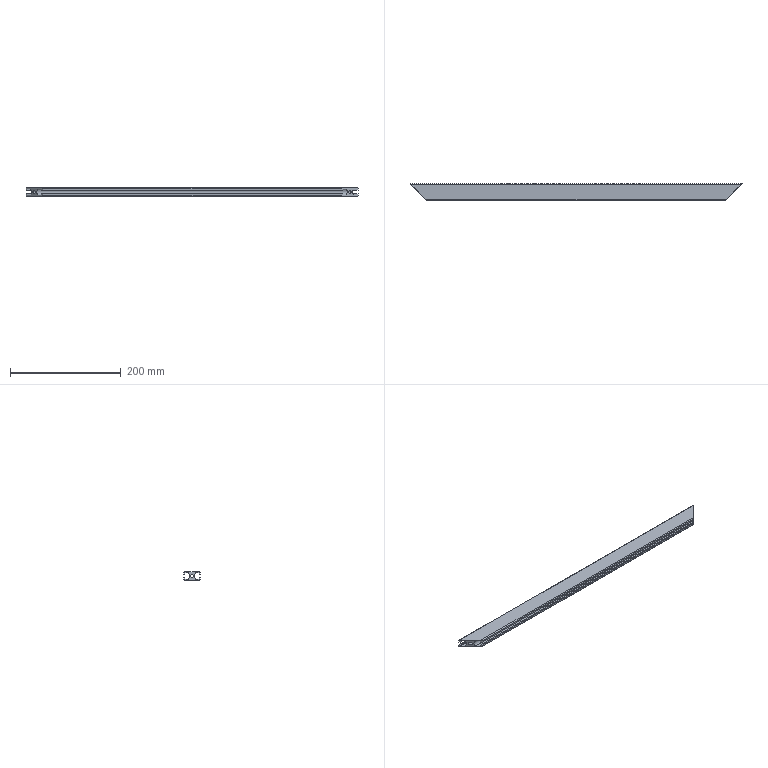Part | SolidWorks | features ICE 2, 3DProfileFeature 1, WeldMemberFeat 1, WeldmentFeature 1 | 1 solid | 31 faces | box 600 x 30 x 15 mm | volume 130266 mm3 | plane 21 | cylinder 10 | commonest cylinder face diameters 3 x4 5 x2 10 x2 15.496 x2
STEP:
#1=CARTESIAN_POINT('',(240.,3.,-2.501));
#2=VERTEX_POINT('',#1);
#3=CARTESIAN_POINT('',(250.,3.,-2.501));
#4=VERTEX_POINT('',#3);
#5=CARTESIAN_POINT('',(245.,3.,-2.501));
#6=DIRECTION('',(0.,0.,1.));
#7=DIRECTION('',(1.,0.,0.));
#8=AXIS2_PLACEMENT_3D('',#5,#6,#7);
#9=CIRCLE('',#8,5.);
#10=EDGE_CURVE('',#2,#4,#9,.T.);
#11=ORIENTED_EDGE('',*,*,#10,.T.);
#12=CARTESIAN_POINT('',(250.,3.,-7.5));
#13=VERTEX_POINT('',#12);
#14=CARTESIAN_POINT('',(250.,3.,-2.501));
#15=DIRECTION('',(0.,0.,-1.));
#16=VECTOR('',#15,1000.);
#17=LINE('',#14,#16);
#18=EDGE_CURVE('',#4,#13,#17,.T.);
#19=ORIENTED_EDGE('',*,*,#18,.T.);
#20=CARTESIAN_POINT('',(240.,3.,-7.5));
#21=VERTEX_POINT('',#20);
#22=CARTESIAN_POINT('',(245.,3.,-7.5));
#23=DIRECTION('',(0.,0.,1.));
#24=DIRECTION('',(1.,0.,0.));
#25=AXIS2_PLACEMENT_3D('',#22,#23,#24);
#26=CIRCLE('',#25,5.);
#27=EDGE_CURVE('',#21,#13,#26,.T.);
#28=ORIENTED_EDGE('',*,*,#27,.F.);
#29=CARTESIAN_POINT('',(240.,3.,-2.501));
#30=DIRECTION('',(0.,0.,-1.));
#31=VECTOR('',#30,1000.);
#32=LINE('',#29,#31);
#33=EDGE_CURVE('',#2,#21,#32,.T.);
#34=ORIENTED_EDGE('',*,*,#33,.F.);
#35=EDGE_LOOP('',(#11,#19,#28,#34));
#36=FACE_OUTER_BOUND('',#35,.T.);
#37=CARTESIAN_POINT('',(245.,3.,-2.501));
#38=DIRECTION('',(0.,0.,-1.));
#39=DIRECTION('',(-1.,0.,0.));
#40=AXIS2_PLACEMENT_3D('',#37,#38,#39);
#41=CYLINDRICAL_SURFACE('',#40,5.);
#42=ADVANCED_FACE('',(#36),#41,.F.);
#43=CARTESIAN_POINT('',(285.,0.,-2.5));
#44=VERTEX_POINT('',#43);
#45=CARTESIAN_POINT('',(285.,0.,2.5));
#46=VERTEX_POINT('',#45);
#47=CARTESIAN_POINT('',(285.,0.,-2.5));
#48=CARTESIAN_POINT('',(280.,-5.,-2.5));
#49=CARTESIAN_POINT('',(280.,-5.,2.5));
#50=CARTESIAN_POINT('',(285.,0.,2.5));
#51=(BOUNDED_CURVE()B_SPLINE_CURVE(3,(#47,#48,#49,#50),.UNSPECIFIED.,.F.,.F.)B_SPLINE_CURVE_WITH_KNOTS((4,4),(4.712,7.854),.UNSPECIFIED.)CURVE()GEOMETRIC_REPRESENTATION_ITEM()RATIONAL_B_SPLINE_CURVE((1.,0.3333,0.3333,1.))REPRESENTATION_ITEM(''));
#52=EDGE_CURVE('',#44,#46,#51,.T.);
#53=ORIENTED_EDGE('',*,*,#52,.F.);
#54=CARTESIAN_POINT('',(-285.,0.,-2.5));
#55=VERTEX_POINT('',#54);
#56=CARTESIAN_POINT('',(300.,0.,-2.5));
#57=DIRECTION('',(-1.,0.,0.));
#58=VECTOR('',#57,1000.);
#59=LINE('',#56,#58);
#60=EDGE_CURVE('',#44,#55,#59,.T.);
#61=ORIENTED_EDGE('',*,*,#60,.T.);
#62=CARTESIAN_POINT('',(-285.,0.,2.5));
#63=VERTEX_POINT('',#62);
#64=CARTESIAN_POINT('',(-285.,0.,2.5));
#65=CARTESIAN_POINT('',(-280.,-5.,2.5));
#66=CARTESIAN_POINT('',(-280.,-5.,-2.5));
#67=CARTESIAN_POINT('',(-285.,0.,-2.5));
#68=(BOUNDED_CURVE()B_SPLINE_CURVE(3,(#64,#65,#66,#67),.UNSPECIFIED.,.F.,.F.)B_SPLINE_CURVE_WITH_KNOTS((4,4),(1.571,4.712),.UNSPECIFIED.)CURVE()GEOMETRIC_REPRESENTATION_ITEM()RATIONAL_B_SPLINE_CURVE((1.,0.3333,0.3333,1.))REPRESENTATION_ITEM(''));
#69=EDGE_CURVE('',#63,#55,#68,.T.);
#70=ORIENTED_EDGE('',*,*,#69,.F.);
#71=CARTESIAN_POINT('',(300.,0.,2.5));
#72=DIRECTION('',(-1.,0.,0.));
#73=VECTOR('',#72,1000.);
#74=LINE('',#71,#73);
#75=EDGE_CURVE('',#46,#63,#74,.T.);
#76=ORIENTED_EDGE('',*,*,#75,.F.);
#77=EDGE_LOOP('',(#53,#61,#70,#76));
#78=FACE_OUTER_BOUND('',#77,.T.);
#79=CARTESIAN_POINT('',(300.,0.,0.));
#80=DIRECTION('',(-1.,0.,0.));
#81=DIRECTION('',(0.,0.,1.));
#82=AXIS2_PLACEMENT_3D('',#79,#80,#81);
#83=CYLINDRICAL_SURFACE('',#82,2.5);
#84=ADVANCED_FACE('',(#78),#83,.F.);
#85=CARTESIAN_POINT('',(298.5,13.5,-7.5));
#86=VERTEX_POINT('',#85);
#87=CARTESIAN_POINT('',(-298.5,13.5,-7.5));
#88=VERTEX_POINT('',#87);
#89=CARTESIAN_POINT('',(300.,13.5,-7.5));
#90=DIRECTION('',(-1.,0.,0.));
#91=VECTOR('',#90,1000.);
#92=LINE('',#89,#91);
#93=EDGE_CURVE('',#86,#88,#92,.T.);
#94=ORIENTED_EDGE('',*,*,#93,.F.);
#95=CARTESIAN_POINT('',(271.5,-13.5,-7.5));
#96=VERTEX_POINT('',#95);
#97=CARTESIAN_POINT('',(300.,15.,-7.5));
#98=DIRECTION('',(-0.7071,-0.7071,0.));
#99=VECTOR('',#98,1000.);
#100=LINE('',#97,#99);
#101=EDGE_CURVE('',#86,#96,#100,.T.);
#102=ORIENTED_EDGE('',*,*,#101,.T.);
#103=CARTESIAN_POINT('',(-271.5,-13.5,-7.5));
#104=VERTEX_POINT('',#103);
#105=CARTESIAN_POINT('',(300.,-13.5,-7.5));
#106=DIRECTION('',(-1.,0.,0.));
#107=VECTOR('',#106,1000.);
#108=LINE('',#105,#107);
#109=EDGE_CURVE('',#96,#104,#108,.T.);
#110=ORIENTED_EDGE('',*,*,#109,.T.);
#111=CARTESIAN_POINT('',(-300.,15.,-7.5));
#112=DIRECTION('',(-0.7071,0.7071,0.));
#113=VECTOR('',#112,1000.);
#114=LINE('',#111,#113);
#115=EDGE_CURVE('',#104,#88,#114,.T.);
#116=ORIENTED_EDGE('',*,*,#115,.T.);
#117=EDGE_LOOP('',(#94,#102,#110,#116));
#118=FACE_OUTER_BOUND('',#117,.T.);
#119=ORIENTED_EDGE('',*,*,#27,.T.);
#120=CARTESIAN_POINT('',(245.,3.,-7.5));
#121=DIRECTION('',(0.,0.,1.));
#122=DIRECTION('',(1.,0.,0.));
#123=AXIS2_PLACEMENT_3D('',#120,#121,#122);
#124=CIRCLE('',#123,5.);
#125=EDGE_CURVE('',#13,#21,#124,.T.);
#126=ORIENTED_EDGE('',*,*,#125,.T.);
#127=EDGE_LOOP('',(#119,#126));
#128=FACE_BOUND('',#127,.T.);
#129=CARTESIAN_POINT('',(300.,-13.5,-7.5));
#130=DIRECTION('',(0.,0.,1.));
#131=DIRECTION('',(1.,0.,0.));
#132=AXIS2_PLACEMENT_3D('',#129,#130,#131);
#133=PLANE('',#132);
#134=ADVANCED_FACE('',(#118,#128),#133,.F.);
#135=CARTESIAN_POINT('',(248.,7.,-5.7));
#136=VERTEX_POINT('',#135);
#137=CARTESIAN_POINT('',(242.,7.,-5.7));
#138=VERTEX_POINT('',#137);
#139=CARTESIAN_POINT('',(245.,3.,-5.7));
#140=DIRECTION('',(0.,0.,1.));
#141=DIRECTION('',(0.,1.,0.));
#142=AXIS2_PLACEMENT_3D('',#139,#140,#141);
#143=CIRCLE('',#142,5.);
#144=EDGE_CURVE('',#136,#138,#143,.T.);
#145=ORIENTED_EDGE('',*,*,#144,.F.);
#146=CARTESIAN_POINT('',(292.,7.,-5.7));
#147=VERTEX_POINT('',#146);
#148=CARTESIAN_POINT('',(300.,7.,-5.7));
#149=DIRECTION('',(-1.,0.,0.));
#150=VECTOR('',#149,1000.);
#151=LINE('',#148,#150);
#152=EDGE_CURVE('',#147,#136,#151,.T.);
#153=ORIENTED_EDGE('',*,*,#152,.F.);
#154=CARTESIAN_POINT('',(297.7,12.7,-5.7));
#155=VERTEX_POINT('',#154);
#156=CARTESIAN_POINT('',(298.85,13.85,-5.7));
#157=DIRECTION('',(0.7071,0.7071,0.));
#158=VECTOR('',#157,1000.);
#159=LINE('',#156,#158);
#160=EDGE_CURVE('',#147,#155,#159,.T.);
#161=ORIENTED_EDGE('',*,*,#160,.T.);
#162=CARTESIAN_POINT('',(-297.7,12.7,-5.7));
#163=VERTEX_POINT('',#162);
#164=CARTESIAN_POINT('',(300.,12.7,-5.7));
#165=DIRECTION('',(-1.,0.,0.));
#166=VECTOR('',#165,1000.);
#167=LINE('',#164,#166);
#168=EDGE_CURVE('',#155,#163,#167,.T.);
#169=ORIENTED_EDGE('',*,*,#168,.T.);
#170=CARTESIAN_POINT('',(-292.,7.,-5.7));
#171=VERTEX_POINT('',#170);
#172=CARTESIAN_POINT('',(1.15,-286.15,-5.7));
#173=DIRECTION('',(0.7071,-0.7071,0.));
#174=VECTOR('',#173,1000.);
#175=LINE('',#172,#174);
#176=EDGE_CURVE('',#163,#171,#175,.T.);
#177=ORIENTED_EDGE('',*,*,#176,.T.);
#178=CARTESIAN_POINT('',(300.,7.,-5.7));
#179=DIRECTION('',(-1.,0.,0.));
#180=VECTOR('',#179,1000.);
#181=LINE('',#178,#180);
#182=EDGE_CURVE('',#138,#171,#181,.T.);
#183=ORIENTED_EDGE('',*,*,#182,.F.);
#184=EDGE_LOOP('',(#145,#153,#161,#169,#177,#183));
#185=FACE_OUTER_BOUND('',#184,.T.);
#186=CARTESIAN_POINT('',(300.,12.7,-5.7));
#187=DIRECTION('',(0.,0.,-1.));
#188=DIRECTION('',(0.,1.,0.));
#189=AXIS2_PLACEMENT_3D('',#186,#187,#188);
#190=PLANE('',#189);
#191=ADVANCED_FACE('',(#185),#190,.F.);
#192=CARTESIAN_POINT('',(240.381,4.915,-2.501));
#193=VERTEX_POINT('',#192);
#194=CARTESIAN_POINT('',(242.,7.,-5.7));
#195=CARTESIAN_POINT('',(241.749,6.812,-5.527));
#196=CARTESIAN_POINT('',(241.535,6.615,-5.328));
#197=CARTESIAN_POINT('',(241.165,6.219,-4.876));
#198=CARTESIAN_POINT('',(241.008,6.019,-4.62));
#199=CARTESIAN_POINT('',(240.753,5.649,-4.073));
#200=CARTESIAN_POINT('',(240.653,5.476,-3.781));
#201=CARTESIAN_POINT('',(240.49,5.165,-3.16));
#202=CARTESIAN_POINT('',(240.429,5.029,-2.836));
#203=CARTESIAN_POINT('',(240.381,4.915,-2.501));
#204=B_SPLINE_CURVE_WITH_KNOTS('',3,(#194,#195,#196,#197,#198,#199,#200,#201,#202,#203),.UNSPECIFIED.,.F.,.F.,(4,2,2,2,4),(0.,0.001057,0.002113,0.00317,0.004226),.UNSPECIFIED.);
#205=EDGE_CURVE('',#138,#193,#204,.T.);
#206=ORIENTED_EDGE('',*,*,#205,.F.);
#207=ORIENTED_EDGE('',*,*,#182,.T.);
#208=CARTESIAN_POINT('',(-292.,7.,5.7));
#209=VERTEX_POINT('',#208);
#210=CARTESIAN_POINT('',(-292.,7.,-5.7));
#211=CARTESIAN_POINT('',(-288.438,3.438,-2.421));
#212=CARTESIAN_POINT('',(-288.438,3.438,2.421));
#213=CARTESIAN_POINT('',(-292.,7.,5.7));
#214=(BOUNDED_CURVE()B_SPLINE_CURVE(3,(#210,#211,#212,#213),.UNSPECIFIED.,.F.,.F.)B_SPLINE_CURVE_WITH_KNOTS((4,4),(2.315,3.968),.UNSPECIFIED.)CURVE()GEOMETRIC_REPRESENTATION_ITEM()RATIONAL_B_SPLINE_CURVE((1.,0.7849,0.7849,1.))REPRESENTATION_ITEM(''));
#215=EDGE_CURVE('',#171,#209,#214,.T.);
#216=ORIENTED_EDGE('',*,*,#215,.T.);
#217=CARTESIAN_POINT('',(292.,7.,5.7));
#218=VERTEX_POINT('',#217);
#219=CARTESIAN_POINT('',(300.,7.,5.7));
#220=DIRECTION('',(-1.,0.,0.));
#221=VECTOR('',#220,1000.);
#222=LINE('',#219,#221);
#223=EDGE_CURVE('',#218,#209,#222,.T.);
#224=ORIENTED_EDGE('',*,*,#223,.F.);
#225=CARTESIAN_POINT('',(292.,7.,5.7));
#226=CARTESIAN_POINT('',(288.438,3.438,2.421));
#227=CARTESIAN_POINT('',(288.438,3.438,-2.421));
#228=CARTESIAN_POINT('',(292.,7.,-5.7));
#229=(BOUNDED_CURVE()B_SPLINE_CURVE(3,(#225,#226,#227,#228),.UNSPECIFIED.,.F.,.F.)B_SPLINE_CURVE_WITH_KNOTS((4,4),(5.457,7.11),.UNSPECIFIED.)CURVE()GEOMETRIC_REPRESENTATION_ITEM()RATIONAL_B_SPLINE_CURVE((1.,0.7849,0.7849,1.))REPRESENTATION_ITEM(''));
#230=EDGE_CURVE('',#218,#147,#229,.T.);
#231=ORIENTED_EDGE('',*,*,#230,.T.);
#232=ORIENTED_EDGE('',*,*,#152,.T.);
#233=CARTESIAN_POINT('',(249.619,4.915,-2.501));
#234=VERTEX_POINT('',#233);
#235=CARTESIAN_POINT('',(249.619,4.915,-2.501));
#236=CARTESIAN_POINT('',(249.572,5.029,-2.836));
#237=CARTESIAN_POINT('',(249.511,5.164,-3.157));
#238=CARTESIAN_POINT('',(249.35,5.471,-3.771));
#239=CARTESIAN_POINT('',(249.25,5.644,-4.066));
#240=CARTESIAN_POINT('',(248.994,6.017,-4.617));
#241=CARTESIAN_POINT('',(248.841,6.213,-4.868));
#242=CARTESIAN_POINT('',(248.47,6.61,-5.323));
#243=CARTESIAN_POINT('',(248.251,6.812,-5.527));
#244=CARTESIAN_POINT('',(248.,7.,-5.7));
#245=B_SPLINE_CURVE_WITH_KNOTS('',3,(#235,#236,#237,#238,#239,#240,#241,#242,#243,#244),.UNSPECIFIED.,.F.,.F.,(4,2,2,2,4),(0.,0.001058,0.002115,0.003173,0.00423),.UNSPECIFIED.);
#246=EDGE_CURVE('',#234,#136,#245,.T.);
#247=ORIENTED_EDGE('',*,*,#246,.F.);
#248=CARTESIAN_POINT('',(300.,4.915,-2.501));
#249=DIRECTION('',(-1.,0.,0.));
#250=VECTOR('',#249,1000.);
#251=LINE('',#248,#250);
#252=EDGE_CURVE('',#234,#193,#251,.T.);
#253=ORIENTED_EDGE('',*,*,#252,.T.);
#254=EDGE_LOOP('',(#206,#207,#216,#224,#231,#232,#247,#253));
#255=FACE_OUTER_BOUND('',#254,.T.);
#256=CARTESIAN_POINT('',(300.,12.248,0.));
#257=DIRECTION('',(-1.,0.,0.));
#258=DIRECTION('',(0.,0.,1.));
#259=AXIS2_PLACEMENT_3D('',#256,#257,#258);
#260=CYLINDRICAL_SURFACE('',#259,7.748);
#261=ADVANCED_FACE('',(#255),#260,.F.);
#262=CARTESIAN_POINT('',(300.,15.,3.25));
#263=VERTEX_POINT('',#262);
#264=CARTESIAN_POINT('',(-300.,15.,3.25));
#265=VERTEX_POINT('',#264);
#266=CARTESIAN_POINT('',(300.,15.,3.25));
#267=DIRECTION('',(-1.,0.,0.));
#268=VECTOR('',#267,1000.);
#269=LINE('',#266,#268);
#270=EDGE_CURVE('',#263,#265,#269,.T.);
#271=ORIENTED_EDGE('',*,*,#270,.F.);
#272=CARTESIAN_POINT('',(297.7,12.7,3.25));
#273=VERTEX_POINT('',#272);
#274=CARTESIAN_POINT('',(300.,15.,3.25));
#275=DIRECTION('',(-0.7071,-0.7071,0.));
#276=VECTOR('',#275,1000.);
#277=LINE('',#274,#276);
#278=EDGE_CURVE('',#263,#273,#277,.T.);
#279=ORIENTED_EDGE('',*,*,#278,.T.);
#280=CARTESIAN_POINT('',(-297.7,12.7,3.25));
#281=VERTEX_POINT('',#280);
#282=CARTESIAN_POINT('',(300.,12.7,3.25));
#283=DIRECTION('',(-1.,0.,0.));
#284=VECTOR('',#283,1000.);
#285=LINE('',#282,#284);
#286=EDGE_CURVE('',#273,#281,#285,.T.);
#287=ORIENTED_EDGE('',*,*,#286,.T.);
#288=CARTESIAN_POINT('',(0.,-285.,3.25));
#289=DIRECTION('',(-0.7071,0.7071,0.));
#290=VECTOR('',#289,1000.);
#291=LINE('',#288,#290);
#292=EDGE_CURVE('',#281,#265,#291,.T.);
#293=ORIENTED_EDGE('',*,*,#292,.T.);
#294=EDGE_LOOP('',(#271,#279,#287,#293));
#295=FACE_OUTER_BOUND('',#294,.T.);
#296=CARTESIAN_POINT('',(300.,15.,3.25));
#297=DIRECTION('',(0.,0.,1.));
#298=DIRECTION('',(0.,-1.,0.));
#299=AXIS2_PLACEMENT_3D('',#296,#297,#298);
#300=PLANE('',#299);
#301=ADVANCED_FACE('',(#295),#300,.F.);
#302=CARTESIAN_POINT('',(-300.,15.,6.));
#303=VERTEX_POINT('',#302);
#304=CARTESIAN_POINT('',(-300.,15.,6.));
#305=DIRECTION('',(0.,0.,1.));
#306=VECTOR('',#305,1000.);
#307=LINE('',#304,#306);
#308=EDGE_CURVE('',#265,#303,#307,.T.);
#309=ORIENTED_EDGE('',*,*,#308,.T.);
#310=CARTESIAN_POINT('',(300.,15.,6.));
#311=VERTEX_POINT('',#310);
#312=CARTESIAN_POINT('',(300.,15.,6.));
#313=DIRECTION('',(-1.,0.,0.));
#314=VECTOR('',#313,1000.);
#315=LINE('',#312,#314);
#316=EDGE_CURVE('',#311,#303,#315,.T.);
#317=ORIENTED_EDGE('',*,*,#316,.F.);
#318=CARTESIAN_POINT('',(300.,15.,6.));
#319=DIRECTION('',(0.,0.,1.));
#320=VECTOR('',#319,1000.);
#321=LINE('',#318,#320);
#322=EDGE_CURVE('',#263,#311,#321,.T.);
#323=ORIENTED_EDGE('',*,*,#322,.F.);
#324=ORIENTED_EDGE('',*,*,#270,.T.);
#325=EDGE_LOOP('',(#309,#317,#323,#324));
#326=FACE_OUTER_BOUND('',#325,.T.);
#327=CARTESIAN_POINT('',(300.,15.,6.));
#328=DIRECTION('',(0.,-1.,0.));
#329=DIRECTION('',(0.,0.,-1.));
#330=AXIS2_PLACEMENT_3D('',#327,#328,#329);
#331=PLANE('',#330);
#332=ADVANCED_FACE('',(#326),#331,.F.);
#333=CARTESIAN_POINT('',(298.5,13.5,7.5));
#334=VERTEX_POINT('',#333);
#335=CARTESIAN_POINT('',(-298.5,13.5,7.5));
#336=VERTEX_POINT('',#335);
#337=CARTESIAN_POINT('',(300.,13.5,7.5));
#338=DIRECTION('',(-1.,0.,0.));
#339=VECTOR('',#338,1000.);
#340=LINE('',#337,#339);
#341=EDGE_CURVE('',#334,#336,#340,.T.);
#342=ORIENTED_EDGE('',*,*,#341,.F.);
#343=CARTESIAN_POINT('',(298.5,13.5,7.5));
#344=CARTESIAN_POINT('',(299.379,14.379,7.5));
#345=CARTESIAN_POINT('',(300.,15.,6.879));
#346=CARTESIAN_POINT('',(300.,15.,6.));
#347=(BOUNDED_CURVE()B_SPLINE_CURVE(3,(#343,#344,#345,#346),.UNSPECIFIED.,.F.,.F.)B_SPLINE_CURVE_WITH_KNOTS((4,4),(1.571,3.142),.UNSPECIFIED.)CURVE()GEOMETRIC_REPRESENTATION_ITEM()RATIONAL_B_SPLINE_CURVE((1.,0.8047,0.8047,1.))REPRESENTATION_ITEM(''));
#348=EDGE_CURVE('',#334,#311,#347,.T.);
#349=ORIENTED_EDGE('',*,*,#348,.T.);
#350=ORIENTED_EDGE('',*,*,#316,.T.);
#351=CARTESIAN_POINT('',(-300.,15.,6.));
#352=CARTESIAN_POINT('',(-300.,15.,6.879));
#353=CARTESIAN_POINT('',(-299.379,14.379,7.5));
#354=CARTESIAN_POINT('',(-298.5,13.5,7.5));
#355=(BOUNDED_CURVE()B_SPLINE_CURVE(3,(#351,#352,#353,#354),.UNSPECIFIED.,.F.,.F.)B_SPLINE_CURVE_WITH_KNOTS((4,4),(0.,1.571),.UNSPECIFIED.)CURVE()GEOMETRIC_REPRESENTATION_ITEM()RATIONAL_B_SPLINE_CURVE((1.,0.8047,0.8047,1.))REPRESENTATION_ITEM(''));
#356=EDGE_CURVE('',#303,#336,#355,.T.);
#357=ORIENTED_EDGE('',*,*,#356,.T.);
#358=EDGE_LOOP('',(#342,#349,#350,#357));
#359=FACE_OUTER_BOUND('',#358,.T.);
#360=CARTESIAN_POINT('',(300.,13.5,6.));
#361=DIRECTION('',(-1.,0.,0.));
#362=DIRECTION('',(0.,0.,1.));
#363=AXIS2_PLACEMENT_3D('',#360,#361,#362);
#364=CYLINDRICAL_SURFACE('',#363,1.5);
#365=ADVANCED_FACE('',(#359),#364,.T.);
#366=CARTESIAN_POINT('',(271.5,-13.5,7.5));
#367=VERTEX_POINT('',#366);
#368=CARTESIAN_POINT('',(-271.5,-13.5,7.5));
#369=VERTEX_POINT('',#368);
#370=CARTESIAN_POINT('',(300.,-13.5,7.5));
#371=DIRECTION('',(-1.,0.,0.));
#372=VECTOR('',#371,1000.);
#373=LINE('',#370,#372);
#374=EDGE_CURVE('',#367,#369,#373,.T.);
#375=ORIENTED_EDGE('',*,*,#374,.F.);
#376=CARTESIAN_POINT('',(300.,15.,7.5));
#377=DIRECTION('',(-0.7071,-0.7071,0.));
#378=VECTOR('',#377,1000.);
#379=LINE('',#376,#378);
#380=EDGE_CURVE('',#334,#367,#379,.T.);
#381=ORIENTED_EDGE('',*,*,#380,.F.);
#382=ORIENTED_EDGE('',*,*,#341,.T.);
#383=CARTESIAN_POINT('',(-300.,15.,7.5));
#384=DIRECTION('',(-0.7071,0.7071,0.));
#385=VECTOR('',#384,1000.);
#386=LINE('',#383,#385);
#387=EDGE_CURVE('',#369,#336,#386,.T.);
#388=ORIENTED_EDGE('',*,*,#387,.F.);
#389=EDGE_LOOP('',(#375,#381,#382,#388));
#390=FACE_OUTER_BOUND('',#389,.T.);
#391=CARTESIAN_POINT('',(300.,-13.5,7.5));
#392=DIRECTION('',(0.,0.,-1.));
#393=DIRECTION('',(-1.,0.,0.));
#394=AXIS2_PLACEMENT_3D('',#391,#392,#393);
#395=PLANE('',#394);
#396=ADVANCED_FACE('',(#390),#395,.F.);
#397=CARTESIAN_POINT('',(270.,-15.,6.));
#398=VERTEX_POINT('',#397);
#399=CARTESIAN_POINT('',(-270.,-15.,6.));
#400=VERTEX_POINT('',#399);
#401=CARTESIAN_POINT('',(300.,-15.,6.));
#402=DIRECTION('',(-1.,0.,0.));
#403=VECTOR('',#402,1000.);
#404=LINE('',#401,#403);
#405=EDGE_CURVE('',#398,#400,#404,.T.);
#406=ORIENTED_EDGE('',*,*,#405,.F.);
#407=CARTESIAN_POINT('',(270.,-15.,6.));
#408=CARTESIAN_POINT('',(270.,-15.,6.879));
#409=CARTESIAN_POINT('',(270.621,-14.379,7.5));
#410=CARTESIAN_POINT('',(271.5,-13.5,7.5));
#411=(BOUNDED_CURVE()B_SPLINE_CURVE(3,(#407,#408,#409,#410),.UNSPECIFIED.,.F.,.F.)B_SPLINE_CURVE_WITH_KNOTS((4,4),(0.,1.571),.UNSPECIFIED.)CURVE()GEOMETRIC_REPRESENTATION_ITEM()RATIONAL_B_SPLINE_CURVE((1.,0.8047,0.8047,1.))REPRESENTATION_ITEM(''));
#412=EDGE_CURVE('',#398,#367,#411,.T.);
#413=ORIENTED_EDGE('',*,*,#412,.T.);
#414=ORIENTED_EDGE('',*,*,#374,.T.);
#415=CARTESIAN_POINT('',(-271.5,-13.5,7.5));
#416=CARTESIAN_POINT('',(-270.621,-14.379,7.5));
#417=CARTESIAN_POINT('',(-270.,-15.,6.879));
#418=CARTESIAN_POINT('',(-270.,-15.,6.));
#419=(BOUNDED_CURVE()B_SPLINE_CURVE(3,(#415,#416,#417,#418),.UNSPECIFIED.,.F.,.F.)B_SPLINE_CURVE_WITH_KNOTS((4,4),(1.571,3.142),.UNSPECIFIED.)CURVE()GEOMETRIC_REPRESENTATION_ITEM()RATIONAL_B_SPLINE_CURVE((1.,0.8047,0.8047,1.))REPRESENTATION_ITEM(''));
#420=EDGE_CURVE('',#369,#400,#419,.T.);
#421=ORIENTED_EDGE('',*,*,#420,.T.);
#422=EDGE_LOOP('',(#406,#413,#414,#421));
#423=FACE_OUTER_BOUND('',#422,.T.);
#424=CARTESIAN_POINT('',(300.,-13.5,6.));
#425=DIRECTION('',(-1.,0.,0.));
#426=DIRECTION('',(0.,0.,1.));
#427=AXIS2_PLACEMENT_3D('',#424,#425,#426);
#428=CYLINDRICAL_SURFACE('',#427,1.5);
#429=ADVANCED_FACE('',(#423),#428,.T.);
#430=CARTESIAN_POINT('',(270.,-15.,3.25));
#431=VERTEX_POINT('',#430);
#432=CARTESIAN_POINT('',(-270.,-15.,3.25));
#433=VERTEX_POINT('',#432);
#434=CARTESIAN_POINT('',(300.,-15.,3.25));
#435=DIRECTION('',(-1.,0.,0.));
#436=VECTOR('',#435,1000.);
#437=LINE('',#434,#436);
#438=EDGE_CURVE('',#431,#433,#437,.T.);
#439=ORIENTED_EDGE('',*,*,#438,.F.);
#440=CARTESIAN_POINT('',(270.,-15.,-7.5));
#441=DIRECTION('',(0.,0.,1.));
#442=VECTOR('',#441,1000.);
#443=LINE('',#440,#442);
#444=EDGE_CURVE('',#431,#398,#443,.T.);
#445=ORIENTED_EDGE('',*,*,#444,.T.);
#446=ORIENTED_EDGE('',*,*,#405,.T.);
#447=CARTESIAN_POINT('',(-270.,-15.,-7.5));
#448=DIRECTION('',(0.,0.,1.));
#449=VECTOR('',#448,1000.);
#450=LINE('',#447,#449);
#451=EDGE_CURVE('',#433,#400,#450,.T.);
#452=ORIENTED_EDGE('',*,*,#451,.F.);
#453=EDGE_LOOP('',(#439,#445,#446,#452));
#454=FACE_OUTER_BOUND('',#453,.T.);
#455=CARTESIAN_POINT('',(300.,-15.,6.));
#456=DIRECTION('',(0.,1.,0.));
#457=DIRECTION('',(0.,0.,1.));
#458=AXIS2_PLACEMENT_3D('',#455,#456,#457);
#459=PLANE('',#458);
#460=ADVANCED_FACE('',(#454),#459,.F.);
#461=CARTESIAN_POINT('',(272.3,-12.7,3.25));
#462=VERTEX_POINT('',#461);
#463=CARTESIAN_POINT('',(-272.3,-12.7,3.25));
#464=VERTEX_POINT('',#463);
#465=CARTESIAN_POINT('',(300.,-12.7,3.25));
#466=DIRECTION('',(-1.,0.,0.));
#467=VECTOR('',#466,1000.);
#468=LINE('',#465,#467);
#469=EDGE_CURVE('',#462,#464,#468,.T.);
#470=ORIENTED_EDGE('',*,*,#469,.F.);
#471=CARTESIAN_POINT('',(285.,0.,3.25));
#472=DIRECTION('',(-0.7071,-0.7071,0.));
#473=VECTOR('',#472,1000.);
#474=LINE('',#471,#473);
#475=EDGE_CURVE('',#462,#431,#474,.T.);
#476=ORIENTED_EDGE('',*,*,#475,.T.);
#477=ORIENTED_EDGE('',*,*,#438,.T.);
#478=CARTESIAN_POINT('',(15.,-300.,3.25));
#479=DIRECTION('',(-0.7071,0.7071,0.));
#480=VECTOR('',#479,1000.);
#481=LINE('',#478,#480);
#482=EDGE_CURVE('',#433,#464,#481,.T.);
#483=ORIENTED_EDGE('',*,*,#482,.T.);
#484=EDGE_LOOP('',(#470,#476,#477,#483));
#485=FACE_OUTER_BOUND('',#484,.T.);
#486=CARTESIAN_POINT('',(300.,-15.,3.25));
#487=DIRECTION('',(0.,0.,1.));
#488=DIRECTION('',(0.,-1.,0.));
#489=AXIS2_PLACEMENT_3D('',#486,#487,#488);
#490=PLANE('',#489);
#491=ADVANCED_FACE('',(#485),#490,.F.);
#492=CARTESIAN_POINT('',(272.3,-12.7,5.7));
#493=VERTEX_POINT('',#492);
#494=CARTESIAN_POINT('',(-272.3,-12.7,5.7));
#495=VERTEX_POINT('',#494);
#496=CARTESIAN_POINT('',(300.,-12.7,5.7));
#497=DIRECTION('',(-1.,0.,0.));
#498=VECTOR('',#497,1000.);
#499=LINE('',#496,#498);
#500=EDGE_CURVE('',#493,#495,#499,.T.);
#501=ORIENTED_EDGE('',*,*,#500,.F.);
#502=CARTESIAN_POINT('',(272.3,-12.7,3.25));
#503=DIRECTION('',(0.,0.,-1.));
#504=VECTOR('',#503,1000.);
#505=LINE('',#502,#504);
#506=EDGE_CURVE('',#493,#462,#505,.T.);
#507=ORIENTED_EDGE('',*,*,#506,.T.);
#508=ORIENTED_EDGE('',*,*,#469,.T.);
#509=CARTESIAN_POINT('',(-272.3,-12.7,3.25));
#510=DIRECTION('',(0.,0.,1.));
#511=VECTOR('',#510,1000.);
#512=LINE('',#509,#511);
#513=EDGE_CURVE('',#464,#495,#512,.T.);
#514=ORIENTED_EDGE('',*,*,#513,.T.);
#515=EDGE_LOOP('',(#501,#507,#508,#514));
#516=FACE_OUTER_BOUND('',#515,.T.);
#517=CARTESIAN_POINT('',(300.,-12.7,3.25));
#518=DIRECTION('',(0.,-1.,0.));
#519=DIRECTION('',(0.,0.,-1.));
#520=AXIS2_PLACEMENT_3D('',#517,#518,#519);
#521=PLANE('',#520);
#522=ADVANCED_FACE('',(#516),#521,.F.);
#523=CARTESIAN_POINT('',(278.,-7.,5.7));
#524=VERTEX_POINT('',#523);
#525=CARTESIAN_POINT('',(-278.,-7.,5.7));
#526=VERTEX_POINT('',#525);
#527=CARTESIAN_POINT('',(300.,-7.,5.7));
#528=DIRECTION('',(-1.,0.,0.));
#529=VECTOR('',#528,1000.);
#530=LINE('',#527,#529);
#531=EDGE_CURVE('',#524,#526,#530,.T.);
#532=ORIENTED_EDGE('',*,*,#531,.F.);
#533=CARTESIAN_POINT('',(286.15,1.15,5.7));
#534=DIRECTION('',(-0.7071,-0.7071,0.));
#535=VECTOR('',#534,1000.);
#536=LINE('',#533,#535);
#537=EDGE_CURVE('',#524,#493,#536,.T.);
#538=ORIENTED_EDGE('',*,*,#537,.T.);
#539=ORIENTED_EDGE('',*,*,#500,.T.);
#540=CARTESIAN_POINT('',(13.85,-298.85,5.7));
#541=DIRECTION('',(-0.7071,0.7071,0.));
#542=VECTOR('',#541,1000.);
#543=LINE('',#540,#542);
#544=EDGE_CURVE('',#495,#526,#543,.T.);
#545=ORIENTED_EDGE('',*,*,#544,.T.);
#546=EDGE_LOOP('',(#532,#538,#539,#545));
#547=FACE_OUTER_BOUND('',#546,.T.);
#548=CARTESIAN_POINT('',(300.,-12.7,5.7));
#549=DIRECTION('',(0.,0.,1.));
#550=DIRECTION('',(0.,-1.,0.));
#551=AXIS2_PLACEMENT_3D('',#548,#549,#550);
#552=PLANE('',#551);
#553=ADVANCED_FACE('',(#547),#552,.F.);
#554=CARTESIAN_POINT('',(278.,-7.,-5.7));
#555=VERTEX_POINT('',#554);
#556=CARTESIAN_POINT('',(-278.,-7.,-5.7));
#557=VERTEX_POINT('',#556);
#558=CARTESIAN_POINT('',(300.,-7.,-5.7));
#559=DIRECTION('',(-1.,0.,0.));
#560=VECTOR('',#559,1000.);
#561=LINE('',#558,#560);
#562=EDGE_CURVE('',#555,#557,#561,.T.);
#563=ORIENTED_EDGE('',*,*,#562,.F.);
#564=CARTESIAN_POINT('',(278.,-7.,-5.7));
#565=CARTESIAN_POINT('',(281.562,-3.438,-2.421));
#566=CARTESIAN_POINT('',(281.562,-3.438,2.421));
#567=CARTESIAN_POINT('',(278.,-7.,5.7));
#568=(BOUNDED_CURVE()B_SPLINE_CURVE(3,(#564,#565,#566,#567),.UNSPECIFIED.,.F.,.F.)B_SPLINE_CURVE_WITH_KNOTS((4,4),(2.315,3.968),.UNSPECIFIED.)CURVE()GEOMETRIC_REPRESENTATION_ITEM()RATIONAL_B_SPLINE_CURVE((1.,0.7849,0.7849,1.))REPRESENTATION_ITEM(''));
#569=EDGE_CURVE('',#555,#524,#568,.T.);
#570=ORIENTED_EDGE('',*,*,#569,.T.);
#571=ORIENTED_EDGE('',*,*,#531,.T.);
#572=CARTESIAN_POINT('',(-278.,-7.,5.7));
#573=CARTESIAN_POINT('',(-281.562,-3.438,2.421));
#574=CARTESIAN_POINT('',(-281.562,-3.438,-2.421));
#575=CARTESIAN_POINT('',(-278.,-7.,-5.7));
#576=(BOUNDED_CURVE()B_SPLINE_CURVE(3,(#572,#573,#574,#575),.UNSPECIFIED.,.F.,.F.)B_SPLINE_CURVE_WITH_KNOTS((4,4),(5.457,7.11),.UNSPECIFIED.)CURVE()GEOMETRIC_REPRESENTATION_ITEM()RATIONAL_B_SPLINE_CURVE((1.,0.7849,0.7849,1.))REPRESENTATION_ITEM(''));
#577=EDGE_CURVE('',#526,#557,#576,.T.);
#578=ORIENTED_EDGE('',*,*,#577,.T.);
#579=EDGE_LOOP('',(#563,#570,#571,#578));
#580=FACE_OUTER_BOUND('',#579,.T.);
#581=CARTESIAN_POINT('',(300.,-12.248,0.));
#582=DIRECTION('',(-1.,0.,0.));
#583=DIRECTION('',(0.,0.,1.));
#584=AXIS2_PLACEMENT_3D('',#581,#582,#583);
#585=CYLINDRICAL_SURFACE('',#584,7.748);
#586=ADVANCED_FACE('',(#580),#585,.F.);
#587=CARTESIAN_POINT('',(272.3,-12.7,-5.7));
#588=VERTEX_POINT('',#587);
#589=CARTESIAN_POINT('',(-272.3,-12.7,-5.7));
#590=VERTEX_POINT('',#589);
#591=CARTESIAN_POINT('',(300.,-12.7,-5.7));
#592=DIRECTION('',(-1.,0.,0.));
#593=VECTOR('',#592,1000.);
#594=LINE('',#591,#593);
#595=EDGE_CURVE('',#588,#590,#594,.T.);
#596=ORIENTED_EDGE('',*,*,#595,.F.);
#597=CARTESIAN_POINT('',(286.15,1.15,-5.7));
#598=DIRECTION('',(0.7071,0.7071,0.));
#599=VECTOR('',#598,1000.);
#600=LINE('',#597,#599);
#601=EDGE_CURVE('',#588,#555,#600,.T.);
#602=ORIENTED_EDGE('',*,*,#601,.T.);
#603=ORIENTED_EDGE('',*,*,#562,.T.);
#604=CARTESIAN_POINT('',(13.85,-298.85,-5.7));
#605=DIRECTION('',(0.7071,-0.7071,0.));
#606=VECTOR('',#605,1000.);
#607=LINE('',#604,#606);
#608=EDGE_CURVE('',#557,#590,#607,.T.);
#609=ORIENTED_EDGE('',*,*,#608,.T.);
#610=EDGE_LOOP('',(#596,#602,#603,#609));
#611=FACE_OUTER_BOUND('',#610,.T.);
#612=CARTESIAN_POINT('',(300.,-12.7,-5.7));
#613=DIRECTION('',(0.,0.,-1.));
#614=DIRECTION('',(0.,1.,0.));
#615=AXIS2_PLACEMENT_3D('',#612,#613,#614);
#616=PLANE('',#615);
#617=ADVANCED_FACE('',(#611),#616,.F.);
#618=CARTESIAN_POINT('',(272.3,-12.7,-3.25));
#619=VERTEX_POINT('',#618);
#620=CARTESIAN_POINT('',(-272.3,-12.7,-3.25));
#621=VERTEX_POINT('',#620);
#622=CARTESIAN_POINT('',(300.,-12.7,-3.25));
#623=DIRECTION('',(-1.,0.,0.));
#624=VECTOR('',#623,1000.);
#625=LINE('',#622,#624);
#626=EDGE_CURVE('',#619,#621,#625,.T.);
#627=ORIENTED_EDGE('',*,*,#626,.F.);
#628=CARTESIAN_POINT('',(272.3,-12.7,-3.25));
#629=DIRECTION('',(0.,0.,-1.));
#630=VECTOR('',#629,1000.);
#631=LINE('',#628,#630);
#632=EDGE_CURVE('',#619,#588,#631,.T.);
#633=ORIENTED_EDGE('',*,*,#632,.T.);
#634=ORIENTED_EDGE('',*,*,#595,.T.);
#635=CARTESIAN_POINT('',(-272.3,-12.7,-3.25));
#636=DIRECTION('',(0.,0.,1.));
#637=VECTOR('',#636,1000.);
#638=LINE('',#635,#637);
#639=EDGE_CURVE('',#590,#621,#638,.T.);
#640=ORIENTED_EDGE('',*,*,#639,.T.);
#641=EDGE_LOOP('',(#627,#633,#634,#640));
#642=FACE_OUTER_BOUND('',#641,.T.);
#643=CARTESIAN_POINT('',(300.,-12.7,-3.25));
#644=DIRECTION('',(0.,-1.,0.));
#645=DIRECTION('',(0.,0.,-1.));
#646=AXIS2_PLACEMENT_3D('',#643,#644,#645);
#647=PLANE('',#646);
#648=ADVANCED_FACE('',(#642),#647,.F.);
#649=CARTESIAN_POINT('',(270.,-15.,-3.25));
#650=VERTEX_POINT('',#649);
#651=CARTESIAN_POINT('',(-270.,-15.,-3.25));
#652=VERTEX_POINT('',#651);
#653=CARTESIAN_POINT('',(300.,-15.,-3.25));
#654=DIRECTION('',(-1.,0.,0.));
#655=VECTOR('',#654,1000.);
#656=LINE('',#653,#655);
#657=EDGE_CURVE('',#650,#652,#656,.T.);
#658=ORIENTED_EDGE('',*,*,#657,.F.);
#659=CARTESIAN_POINT('',(285.,0.,-3.25));
#660=DIRECTION('',(0.7071,0.7071,0.));
#661=VECTOR('',#660,1000.);
#662=LINE('',#659,#661);
#663=EDGE_CURVE('',#650,#619,#662,.T.);
#664=ORIENTED_EDGE('',*,*,#663,.T.);
#665=ORIENTED_EDGE('',*,*,#626,.T.);
#666=CARTESIAN_POINT('',(15.,-300.,-3.25));
#667=DIRECTION('',(0.7071,-0.7071,0.));
#668=VECTOR('',#667,1000.);
#669=LINE('',#666,#668);
#670=EDGE_CURVE('',#621,#652,#669,.T.);
#671=ORIENTED_EDGE('',*,*,#670,.T.);
#672=EDGE_LOOP('',(#658,#664,#665,#671));
#673=FACE_OUTER_BOUND('',#672,.T.);
#674=CARTESIAN_POINT('',(300.,-15.,-3.25));
#675=DIRECTION('',(0.,0.,-1.));
#676=DIRECTION('',(0.,1.,0.));
#677=AXIS2_PLACEMENT_3D('',#674,#675,#676);
#678=PLANE('',#677);
#679=ADVANCED_FACE('',(#673),#678,.F.);
#680=CARTESIAN_POINT('',(270.,-15.,-6.));
#681=VERTEX_POINT('',#680);
#682=CARTESIAN_POINT('',(-270.,-15.,-6.));
#683=VERTEX_POINT('',#682);
#684=CARTESIAN_POINT('',(300.,-15.,-6.));
#685=DIRECTION('',(-1.,0.,0.));
#686=VECTOR('',#685,1000.);
#687=LINE('',#684,#686);
#688=EDGE_CURVE('',#681,#683,#687,.T.);
#689=ORIENTED_EDGE('',*,*,#688,.F.);
#690=CARTESIAN_POINT('',(270.,-15.,-7.5));
#691=DIRECTION('',(0.,0.,1.));
#692=VECTOR('',#691,1000.);
#693=LINE('',#690,#692);
#694=EDGE_CURVE('',#681,#650,#693,.T.);
#695=ORIENTED_EDGE('',*,*,#694,.T.);
#696=ORIENTED_EDGE('',*,*,#657,.T.);
#697=CARTESIAN_POINT('',(-270.,-15.,-7.5));
#698=DIRECTION('',(0.,0.,1.));
#699=VECTOR('',#698,1000.);
#700=LINE('',#697,#699);
#701=EDGE_CURVE('',#683,#652,#700,.T.);
#702=ORIENTED_EDGE('',*,*,#701,.F.);
#703=EDGE_LOOP('',(#689,#695,#696,#702));
#704=FACE_OUTER_BOUND('',#703,.T.);
#705=CARTESIAN_POINT('',(300.,-15.,-3.25));
#706=DIRECTION('',(0.,1.,0.));
#707=DIRECTION('',(0.,0.,1.));
#708=AXIS2_PLACEMENT_3D('',#705,#706,#707);
#709=PLANE('',#708);
#710=ADVANCED_FACE('',(#704),#709,.F.);
#711=ORIENTED_EDGE('',*,*,#109,.F.);
#712=CARTESIAN_POINT('',(271.5,-13.5,-7.5));
#713=CARTESIAN_POINT('',(270.621,-14.379,-7.5));
#714=CARTESIAN_POINT('',(270.,-15.,-6.879));
#715=CARTESIAN_POINT('',(270.,-15.,-6.));
#716=(BOUNDED_CURVE()B_SPLINE_CURVE(3,(#712,#713,#714,#715),.UNSPECIFIED.,.F.,.F.)B_SPLINE_CURVE_WITH_KNOTS((4,4),(4.712,6.283),.UNSPECIFIED.)CURVE()GEOMETRIC_REPRESENTATION_ITEM()RATIONAL_B_SPLINE_CURVE((1.,0.8047,0.8047,1.))REPRESENTATION_ITEM(''));
#717=EDGE_CURVE('',#96,#681,#716,.T.);
#718=ORIENTED_EDGE('',*,*,#717,.T.);
#719=ORIENTED_EDGE('',*,*,#688,.T.);
#720=CARTESIAN_POINT('',(-270.,-15.,-6.));
#721=CARTESIAN_POINT('',(-270.,-15.,-6.879));
#722=CARTESIAN_POINT('',(-270.621,-14.379,-7.5));
#723=CARTESIAN_POINT('',(-271.5,-13.5,-7.5));
#724=(BOUNDED_CURVE()B_SPLINE_CURVE(3,(#720,#721,#722,#723),.UNSPECIFIED.,.F.,.F.)B_SPLINE_CURVE_WITH_KNOTS((4,4),(3.142,4.712),.UNSPECIFIED.)CURVE()GEOMETRIC_REPRESENTATION_ITEM()RATIONAL_B_SPLINE_CURVE((1.,0.8047,0.8047,1.))REPRESENTATION_ITEM(''));
#725=EDGE_CURVE('',#683,#104,#724,.T.);
#726=ORIENTED_EDGE('',*,*,#725,.T.);
#727=EDGE_LOOP('',(#711,#718,#719,#726));
#728=FACE_OUTER_BOUND('',#727,.T.);
#729=CARTESIAN_POINT('',(300.,-13.5,-6.));
#730=DIRECTION('',(-1.,0.,0.));
#731=DIRECTION('',(0.,0.,1.));
#732=AXIS2_PLACEMENT_3D('',#729,#730,#731);
#733=CYLINDRICAL_SURFACE('',#732,1.5);
#734=ADVANCED_FACE('',(#728),#733,.T.);
#735=CARTESIAN_POINT('',(300.,15.,-6.));
#736=VERTEX_POINT('',#735);
#737=CARTESIAN_POINT('',(-300.,15.,-6.));
#738=VERTEX_POINT('',#737);
#739=CARTESIAN_POINT('',(300.,15.,-6.));
#740=DIRECTION('',(-1.,0.,0.));
#741=VECTOR('',#740,1000.);
#742=LINE('',#739,#741);
#743=EDGE_CURVE('',#736,#738,#742,.T.);
#744=ORIENTED_EDGE('',*,*,#743,.F.);
#745=CARTESIAN_POINT('',(300.,15.,-6.));
#746=CARTESIAN_POINT('',(300.,15.,-6.879));
#747=CARTESIAN_POINT('',(299.379,14.379,-7.5));
#748=CARTESIAN_POINT('',(298.5,13.5,-7.5));
#749=(BOUNDED_CURVE()B_SPLINE_CURVE(3,(#745,#746,#747,#748),.UNSPECIFIED.,.F.,.F.)B_SPLINE_CURVE_WITH_KNOTS((4,4),(3.142,4.712),.UNSPECIFIED.)CURVE()GEOMETRIC_REPRESENTATION_ITEM()RATIONAL_B_SPLINE_CURVE((1.,0.8047,0.8047,1.))REPRESENTATION_ITEM(''));
#750=EDGE_CURVE('',#736,#86,#749,.T.);
#751=ORIENTED_EDGE('',*,*,#750,.T.);
#752=ORIENTED_EDGE('',*,*,#93,.T.);
#753=CARTESIAN_POINT('',(-298.5,13.5,-7.5));
#754=CARTESIAN_POINT('',(-299.379,14.379,-7.5));
#755=CARTESIAN_POINT('',(-300.,15.,-6.879));
#756=CARTESIAN_POINT('',(-300.,15.,-6.));
#757=(BOUNDED_CURVE()B_SPLINE_CURVE(3,(#753,#754,#755,#756),.UNSPECIFIED.,.F.,.F.)B_SPLINE_CURVE_WITH_KNOTS((4,4),(4.712,6.283),.UNSPECIFIED.)CURVE()GEOMETRIC_REPRESENTATION_ITEM()RATIONAL_B_SPLINE_CURVE((1.,0.8047,0.8047,1.))REPRESENTATION_ITEM(''));
#758=EDGE_CURVE('',#88,#738,#757,.T.);
#759=ORIENTED_EDGE('',*,*,#758,.T.);
#760=EDGE_LOOP('',(#744,#751,#752,#759));
#761=FACE_OUTER_BOUND('',#760,.T.);
#762=CARTESIAN_POINT('',(300.,13.5,-6.));
#763=DIRECTION('',(-1.,0.,0.));
#764=DIRECTION('',(0.,0.,1.));
#765=AXIS2_PLACEMENT_3D('',#762,#763,#764);
#766=CYLINDRICAL_SURFACE('',#765,1.5);
#767=ADVANCED_FACE('',(#761),#766,.T.);
#768=CARTESIAN_POINT('',(-300.,15.,-3.25));
#769=VERTEX_POINT('',#768);
#770=CARTESIAN_POINT('',(-300.,15.,-3.25));
#771=DIRECTION('',(0.,0.,1.));
#772=VECTOR('',#771,1000.);
#773=LINE('',#770,#772);
#774=EDGE_CURVE('',#738,#769,#773,.T.);
#775=ORIENTED_EDGE('',*,*,#774,.T.);
#776=CARTESIAN_POINT('',(300.,15.,-3.25));
#777=VERTEX_POINT('',#776);
#778=CARTESIAN_POINT('',(300.,15.,-3.25));
#779=DIRECTION('',(-1.,0.,0.));
#780=VECTOR('',#779,1000.);
#781=LINE('',#778,#780);
#782=EDGE_CURVE('',#777,#769,#781,.T.);
#783=ORIENTED_EDGE('',*,*,#782,.F.);
#784=CARTESIAN_POINT('',(300.,15.,-3.25));
#785=DIRECTION('',(0.,0.,1.));
#786=VECTOR('',#785,1000.);
#787=LINE('',#784,#786);
#788=EDGE_CURVE('',#736,#777,#787,.T.);
#789=ORIENTED_EDGE('',*,*,#788,.F.);
#790=ORIENTED_EDGE('',*,*,#743,.T.);
#791=EDGE_LOOP('',(#775,#783,#789,#790));
#792=FACE_OUTER_BOUND('',#791,.T.);
#793=CARTESIAN_POINT('',(300.,15.,-3.25));
#794=DIRECTION('',(0.,-1.,0.));
#795=DIRECTION('',(0.,0.,-1.));
#796=AXIS2_PLACEMENT_3D('',#793,#794,#795);
#797=PLANE('',#796);
#798=ADVANCED_FACE('',(#792),#797,.F.);
#799=CARTESIAN_POINT('',(297.7,12.7,-3.25));
#800=VERTEX_POINT('',#799);
#801=CARTESIAN_POINT('',(-297.7,12.7,-3.25));
#802=VERTEX_POINT('',#801);
#803=CARTESIAN_POINT('',(300.,12.7,-3.25));
#804=DIRECTION('',(-1.,0.,0.));
#805=VECTOR('',#804,1000.);
#806=LINE('',#803,#805);
#807=EDGE_CURVE('',#800,#802,#806,.T.);
#808=ORIENTED_EDGE('',*,*,#807,.F.);
#809=CARTESIAN_POINT('',(300.,15.,-3.25));
#810=DIRECTION('',(0.7071,0.7071,0.));
#811=VECTOR('',#810,1000.);
#812=LINE('',#809,#811);
#813=EDGE_CURVE('',#800,#777,#812,.T.);
#814=ORIENTED_EDGE('',*,*,#813,.T.);
#815=ORIENTED_EDGE('',*,*,#782,.T.);
#816=CARTESIAN_POINT('',(0.,-285.,-3.25));
#817=DIRECTION('',(0.7071,-0.7071,0.));
#818=VECTOR('',#817,1000.);
#819=LINE('',#816,#818);
#820=EDGE_CURVE('',#769,#802,#819,.T.);
#821=ORIENTED_EDGE('',*,*,#820,.T.);
#822=EDGE_LOOP('',(#808,#814,#815,#821));
#823=FACE_OUTER_BOUND('',#822,.T.);
#824=CARTESIAN_POINT('',(300.,15.,-3.25));
#825=DIRECTION('',(0.,0.,-1.));
#826=DIRECTION('',(0.,1.,0.));
#827=AXIS2_PLACEMENT_3D('',#824,#825,#826);
#828=PLANE('',#827);
#829=ADVANCED_FACE('',(#823),#828,.F.);
#830=ORIENTED_EDGE('',*,*,#168,.F.);
#831=CARTESIAN_POINT('',(297.7,12.7,-3.25));
#832=DIRECTION('',(0.,0.,1.));
#833=VECTOR('',#832,1000.);
#834=LINE('',#831,#833);
#835=EDGE_CURVE('',#155,#800,#834,.T.);
#836=ORIENTED_EDGE('',*,*,#835,.T.);
#837=ORIENTED_EDGE('',*,*,#807,.T.);
#838=CARTESIAN_POINT('',(-297.7,12.7,-3.25));
#839=DIRECTION('',(0.,0.,-1.));
#840=VECTOR('',#839,1000.);
#841=LINE('',#838,#840);
#842=EDGE_CURVE('',#802,#163,#841,.T.);
#843=ORIENTED_EDGE('',*,*,#842,.T.);
#844=EDGE_LOOP('',(#830,#836,#837,#843));
#845=FACE_OUTER_BOUND('',#844,.T.);
#846=CARTESIAN_POINT('',(300.,12.7,-3.25));
#847=DIRECTION('',(0.,1.,0.));
#848=DIRECTION('',(0.,0.,1.));
#849=AXIS2_PLACEMENT_3D('',#846,#847,#848);
#850=PLANE('',#849);
#851=ADVANCED_FACE('',(#845),#850,.F.);
#852=CARTESIAN_POINT('',(297.7,12.7,5.7));
#853=VERTEX_POINT('',#852);
#854=CARTESIAN_POINT('',(-297.7,12.7,5.7));
#855=VERTEX_POINT('',#854);
#856=CARTESIAN_POINT('',(300.,12.7,5.7));
#857=DIRECTION('',(-1.,0.,0.));
#858=VECTOR('',#857,1000.);
#859=LINE('',#856,#858);
#860=EDGE_CURVE('',#853,#855,#859,.T.);
#861=ORIENTED_EDGE('',*,*,#860,.F.);
#862=CARTESIAN_POINT('',(298.85,13.85,5.7));
#863=DIRECTION('',(-0.7071,-0.7071,0.));
#864=VECTOR('',#863,1000.);
#865=LINE('',#862,#864);
#866=EDGE_CURVE('',#853,#218,#865,.T.);
#867=ORIENTED_EDGE('',*,*,#866,.T.);
#868=ORIENTED_EDGE('',*,*,#223,.T.);
#869=CARTESIAN_POINT('',(1.15,-286.15,5.7));
#870=DIRECTION('',(-0.7071,0.7071,0.));
#871=VECTOR('',#870,1000.);
#872=LINE('',#869,#871);
#873=EDGE_CURVE('',#209,#855,#872,.T.);
#874=ORIENTED_EDGE('',*,*,#873,.T.);
#875=EDGE_LOOP('',(#861,#867,#868,#874));
#876=FACE_OUTER_BOUND('',#875,.T.);
#877=CARTESIAN_POINT('',(300.,12.7,5.7));
#878=DIRECTION('',(0.,0.,1.));
#879=DIRECTION('',(0.,-1.,0.));
#880=AXIS2_PLACEMENT_3D('',#877,#878,#879);
#881=PLANE('',#880);
#882=ADVANCED_FACE('',(#876),#881,.F.);
#883=ORIENTED_EDGE('',*,*,#60,.F.);
#884=CARTESIAN_POINT('',(285.,0.,2.5));
#885=CARTESIAN_POINT('',(290.,5.,2.5));
#886=CARTESIAN_POINT('',(290.,5.,-2.5));
#887=CARTESIAN_POINT('',(285.,0.,-2.5));
#888=(BOUNDED_CURVE()B_SPLINE_CURVE(3,(#884,#885,#886,#887),.UNSPECIFIED.,.F.,.F.)B_SPLINE_CURVE_WITH_KNOTS((4,4),(1.571,4.712),.UNSPECIFIED.)CURVE()GEOMETRIC_REPRESENTATION_ITEM()RATIONAL_B_SPLINE_CURVE((1.,0.3333,0.3333,1.))REPRESENTATION_ITEM(''));
#889=EDGE_CURVE('',#46,#44,#888,.T.);
#890=ORIENTED_EDGE('',*,*,#889,.F.);
#891=ORIENTED_EDGE('',*,*,#75,.T.);
#892=CARTESIAN_POINT('',(-285.,0.,-2.5));
#893=CARTESIAN_POINT('',(-290.,5.,-2.5));
#894=CARTESIAN_POINT('',(-290.,5.,2.5));
#895=CARTESIAN_POINT('',(-285.,0.,2.5));
#896=(BOUNDED_CURVE()B_SPLINE_CURVE(3,(#892,#893,#894,#895),.UNSPECIFIED.,.F.,.F.)B_SPLINE_CURVE_WITH_KNOTS((4,4),(4.712,7.854),.UNSPECIFIED.)CURVE()GEOMETRIC_REPRESENTATION_ITEM()RATIONAL_B_SPLINE_CURVE((1.,0.3333,0.3333,1.))REPRESENTATION_ITEM(''));
#897=EDGE_CURVE('',#55,#63,#896,.T.);
#898=ORIENTED_EDGE('',*,*,#897,.F.);
#899=EDGE_LOOP('',(#883,#890,#891,#898));
#900=FACE_OUTER_BOUND('',#899,.T.);
#901=CARTESIAN_POINT('',(300.,0.,0.));
#902=DIRECTION('',(-1.,0.,0.));
#903=DIRECTION('',(0.,0.,1.));
#904=AXIS2_PLACEMENT_3D('',#901,#902,#903);
#905=CYLINDRICAL_SURFACE('',#904,2.5);
#906=ADVANCED_FACE('',(#900),#905,.F.);
#907=ORIENTED_EDGE('',*,*,#286,.F.);
#908=CARTESIAN_POINT('',(297.7,12.7,3.25));
#909=DIRECTION('',(0.,0.,1.));
#910=VECTOR('',#909,1000.);
#911=LINE('',#908,#910);
#912=EDGE_CURVE('',#273,#853,#911,.T.);
#913=ORIENTED_EDGE('',*,*,#912,.T.);
#914=ORIENTED_EDGE('',*,*,#860,.T.);
#915=CARTESIAN_POINT('',(-297.7,12.7,3.25));
#916=DIRECTION('',(0.,0.,-1.));
#917=VECTOR('',#916,1000.);
#918=LINE('',#915,#917);
#919=EDGE_CURVE('',#855,#281,#918,.T.);
#920=ORIENTED_EDGE('',*,*,#919,.T.);
#921=EDGE_LOOP('',(#907,#913,#914,#920));
#922=FACE_OUTER_BOUND('',#921,.T.);
#923=CARTESIAN_POINT('',(300.,12.7,3.25));
#924=DIRECTION('',(0.,1.,0.));
#925=DIRECTION('',(0.,0.,1.));
#926=AXIS2_PLACEMENT_3D('',#923,#924,#925);
#927=PLANE('',#926);
#928=ADVANCED_FACE('',(#922),#927,.F.);
#929=ORIENTED_EDGE('',*,*,#69,.T.);
#930=ORIENTED_EDGE('',*,*,#897,.T.);
#931=EDGE_LOOP('',(#929,#930));
#932=FACE_BOUND('',#931,.T.);
#933=ORIENTED_EDGE('',*,*,#308,.F.);
#934=ORIENTED_EDGE('',*,*,#292,.F.);
#935=ORIENTED_EDGE('',*,*,#919,.F.);
#936=ORIENTED_EDGE('',*,*,#873,.F.);
#937=ORIENTED_EDGE('',*,*,#215,.F.);
#938=ORIENTED_EDGE('',*,*,#176,.F.);
#939=ORIENTED_EDGE('',*,*,#842,.F.);
#940=ORIENTED_EDGE('',*,*,#820,.F.);
#941=ORIENTED_EDGE('',*,*,#774,.F.);
#942=ORIENTED_EDGE('',*,*,#758,.F.);
#943=ORIENTED_EDGE('',*,*,#115,.F.);
#944=ORIENTED_EDGE('',*,*,#725,.F.);
#945=ORIENTED_EDGE('',*,*,#701,.T.);
#946=ORIENTED_EDGE('',*,*,#670,.F.);
#947=ORIENTED_EDGE('',*,*,#639,.F.);
#948=ORIENTED_EDGE('',*,*,#608,.F.);
#949=ORIENTED_EDGE('',*,*,#577,.F.);
#950=ORIENTED_EDGE('',*,*,#544,.F.);
#951=ORIENTED_EDGE('',*,*,#513,.F.);
#952=ORIENTED_EDGE('',*,*,#482,.F.);
#953=ORIENTED_EDGE('',*,*,#451,.T.);
#954=ORIENTED_EDGE('',*,*,#420,.F.);
#955=ORIENTED_EDGE('',*,*,#387,.T.);
#956=ORIENTED_EDGE('',*,*,#356,.F.);
#957=EDGE_LOOP('',(#933,#934,#935,#936,#937,#938,#939,#940,#941,#942,#943,#944,#945,#946,#947,#948,#949,#950,#951,#952,#953,#954,#955,#956));
#958=FACE_OUTER_BOUND('',#957,.T.);
#959=CARTESIAN_POINT('',(-300.,15.,-7.5));
#960=DIRECTION('',(0.7071,0.7071,0.));
#961=DIRECTION('',(-0.7071,0.7071,0.));
#962=AXIS2_PLACEMENT_3D('',#959,#960,#961);
#963=PLANE('',#962);
#964=ADVANCED_FACE('',(#932,#958),#963,.F.);
#965=ORIENTED_EDGE('',*,*,#889,.T.);
#966=ORIENTED_EDGE('',*,*,#52,.T.);
#967=EDGE_LOOP('',(#965,#966));
#968=FACE_BOUND('',#967,.T.);
#969=ORIENTED_EDGE('',*,*,#380,.T.);
#970=ORIENTED_EDGE('',*,*,#412,.F.);
#971=ORIENTED_EDGE('',*,*,#444,.F.);
#972=ORIENTED_EDGE('',*,*,#475,.F.);
#973=ORIENTED_EDGE('',*,*,#506,.F.);
#974=ORIENTED_EDGE('',*,*,#537,.F.);
#975=ORIENTED_EDGE('',*,*,#569,.F.);
#976=ORIENTED_EDGE('',*,*,#601,.F.);
#977=ORIENTED_EDGE('',*,*,#632,.F.);
#978=ORIENTED_EDGE('',*,*,#663,.F.);
#979=ORIENTED_EDGE('',*,*,#694,.F.);
#980=ORIENTED_EDGE('',*,*,#717,.F.);
#981=ORIENTED_EDGE('',*,*,#101,.F.);
#982=ORIENTED_EDGE('',*,*,#750,.F.);
#983=ORIENTED_EDGE('',*,*,#788,.T.);
#984=ORIENTED_EDGE('',*,*,#813,.F.);
#985=ORIENTED_EDGE('',*,*,#835,.F.);
#986=ORIENTED_EDGE('',*,*,#160,.F.);
#987=ORIENTED_EDGE('',*,*,#230,.F.);
#988=ORIENTED_EDGE('',*,*,#866,.F.);
#989=ORIENTED_EDGE('',*,*,#912,.F.);
#990=ORIENTED_EDGE('',*,*,#278,.F.);
#991=ORIENTED_EDGE('',*,*,#322,.T.);
#992=ORIENTED_EDGE('',*,*,#348,.F.);
#993=EDGE_LOOP('',(#969,#970,#971,#972,#973,#974,#975,#976,#977,#978,#979,#980,#981,#982,#983,#984,#985,#986,#987,#988,#989,#990,#991,#992));
#994=FACE_OUTER_BOUND('',#993,.T.);
#995=CARTESIAN_POINT('',(300.,15.,-7.5));
#996=DIRECTION('',(-0.7071,0.7071,0.));
#997=DIRECTION('',(-0.7071,-0.7071,0.));
#998=AXIS2_PLACEMENT_3D('',#995,#996,#997);
#999=PLANE('',#998);
#1000=ADVANCED_FACE('',(#968,#994),#999,.F.);
#1001=ORIENTED_EDGE('',*,*,#18,.F.);
#1002=CARTESIAN_POINT('',(245.,3.,-2.501));
#1003=DIRECTION('',(0.,0.,1.));
#1004=DIRECTION('',(1.,0.,0.));
#1005=AXIS2_PLACEMENT_3D('',#1002,#1003,#1004);
#1006=CIRCLE('',#1005,5.);
#1007=EDGE_CURVE('',#4,#234,#1006,.T.);
#1008=ORIENTED_EDGE('',*,*,#1007,.T.);
#1009=ORIENTED_EDGE('',*,*,#246,.T.);
#1010=ORIENTED_EDGE('',*,*,#144,.T.);
#1011=ORIENTED_EDGE('',*,*,#205,.T.);
#1012=CARTESIAN_POINT('',(245.,3.,-2.501));
#1013=DIRECTION('',(0.,0.,1.));
#1014=DIRECTION('',(1.,0.,0.));
#1015=AXIS2_PLACEMENT_3D('',#1012,#1013,#1014);
#1016=CIRCLE('',#1015,5.);
#1017=EDGE_CURVE('',#193,#2,#1016,.T.);
#1018=ORIENTED_EDGE('',*,*,#1017,.T.);
#1019=ORIENTED_EDGE('',*,*,#33,.T.);
#1020=ORIENTED_EDGE('',*,*,#125,.F.);
#1021=EDGE_LOOP('',(#1001,#1008,#1009,#1010,#1011,#1018,#1019,#1020));
#1022=FACE_OUTER_BOUND('',#1021,.T.);
#1023=CARTESIAN_POINT('',(245.,3.,-2.501));
#1024=DIRECTION('',(0.,0.,-1.));
#1025=DIRECTION('',(-1.,0.,0.));
#1026=AXIS2_PLACEMENT_3D('',#1023,#1024,#1025);
#1027=CYLINDRICAL_SURFACE('',#1026,5.);
#1028=ADVANCED_FACE('',(#1022),#1027,.F.);
#1029=ORIENTED_EDGE('',*,*,#1017,.F.);
#1030=ORIENTED_EDGE('',*,*,#252,.F.);
#1031=ORIENTED_EDGE('',*,*,#1007,.F.);
#1032=ORIENTED_EDGE('',*,*,#10,.F.);
#1033=EDGE_LOOP('',(#1029,#1030,#1031,#1032));
#1034=FACE_OUTER_BOUND('',#1033,.T.);
#1035=CARTESIAN_POINT('',(245.,3.,-2.501));
#1036=DIRECTION('',(0.,0.,1.));
#1037=DIRECTION('',(1.,0.,0.));
#1038=AXIS2_PLACEMENT_3D('',#1035,#1036,#1037);
#1039=PLANE('',#1038);
#1040=ADVANCED_FACE('',(#1034),#1039,.F.);
#1041=CLOSED_SHELL('',(#42,#84,#134,#191,#261,#301,#332,#365,#396,#429,#460,#491,#522,#553,#586,#617,#648,#679,#710,#734,#767,#798,#829,#851,#882,#906,#928,#964,#1000,#1028,#1040));
#1042=MANIFOLD_SOLID_BREP('',#1041);
#1043=CARTESIAN_POINT('',(0.,0.,0.));
#1044=DIRECTION('',(0.,0.,1.));
#1045=DIRECTION('',(1.,0.,0.));
#1046=AXIS2_PLACEMENT_3D('',#1043,#1044,#1045);
#1047=(LENGTH_UNIT()NAMED_UNIT(*)SI_UNIT(.MILLI.,.METRE.));
#1048=UNCERTAINTY_MEASURE_WITH_UNIT(LENGTH_MEASURE(0.00001),#1047,'','');
#1049=(NAMED_UNIT(*)PLANE_ANGLE_UNIT()SI_UNIT($,.RADIAN.));
#1050=(NAMED_UNIT(*)SI_UNIT($,.STERADIAN.)SOLID_ANGLE_UNIT());
#1051=(GEOMETRIC_REPRESENTATION_CONTEXT(3)GLOBAL_UNCERTAINTY_ASSIGNED_CONTEXT((#1048))GLOBAL_UNIT_ASSIGNED_CONTEXT((#1047,#1049,#1050))REPRESENTATION_CONTEXT('',''));
#1052=ADVANCED_BREP_SHAPE_REPRESENTATION('',(#1042,#1046),#1051);